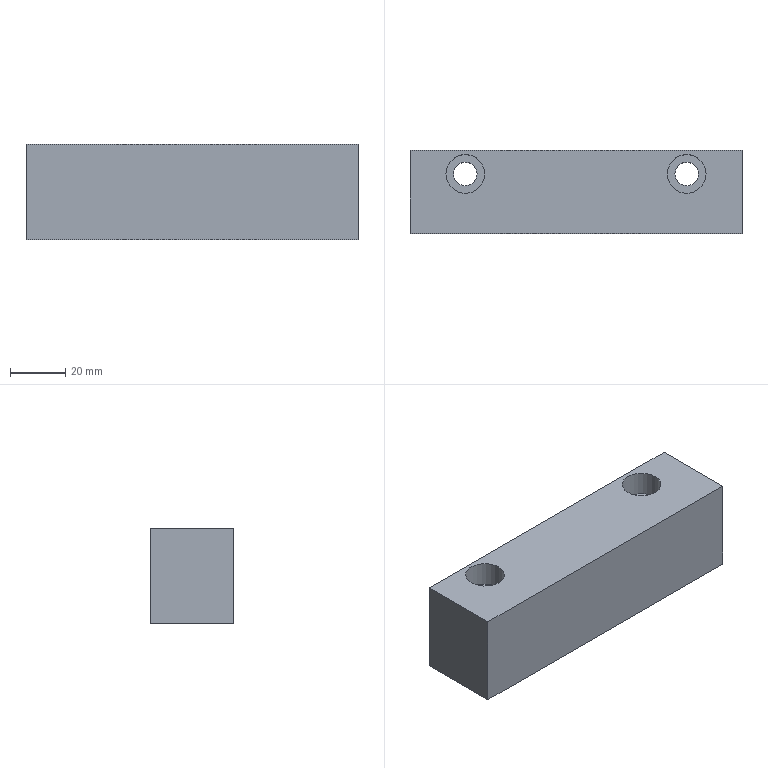Part | NX | features solid 2 | 1 solid | 12 faces | box 120 x 30 x 34.5 mm | volume 118535 mm3 | plane 8 | cylinder 4 | commonest cylinder face diameters 8.5 x2 14 x2
STEP:
#1=CARTESIAN_POINT('',(-55.,85.,-35.));
#2=VERTEX_POINT('',#1);
#3=CARTESIAN_POINT('',(-55.,115.,-35.));
#4=VERTEX_POINT('',#3);
#5=CARTESIAN_POINT('',(-55.,92.5,-35.));
#6=DIRECTION('',(0.,1.,0.));
#7=VECTOR('',#6,1000.);
#8=LINE('',#5,#7);
#9=EDGE_CURVE('',#2,#4,#8,.T.);
#10=ORIENTED_EDGE('',*,*,#9,.F.);
#11=CARTESIAN_POINT('',(-175.,85.,-35.));
#12=VERTEX_POINT('',#11);
#13=CARTESIAN_POINT('',(-90.,85.,-35.));
#14=DIRECTION('',(1.,0.,0.));
#15=VECTOR('',#14,1000.);
#16=LINE('',#13,#15);
#17=EDGE_CURVE('',#12,#2,#16,.T.);
#18=ORIENTED_EDGE('',*,*,#17,.F.);
#19=CARTESIAN_POINT('',(-175.,115.,-35.));
#20=VERTEX_POINT('',#19);
#21=CARTESIAN_POINT('',(-175.,0.,-35.));
#22=DIRECTION('',(0.,-1.,0.));
#23=VECTOR('',#22,1000.);
#24=LINE('',#21,#23);
#25=EDGE_CURVE('',#20,#12,#24,.T.);
#26=ORIENTED_EDGE('',*,*,#25,.F.);
#27=CARTESIAN_POINT('',(-90.,115.,-35.));
#28=DIRECTION('',(-1.,0.,0.));
#29=VECTOR('',#28,1000.);
#30=LINE('',#27,#29);
#31=EDGE_CURVE('',#4,#20,#30,.T.);
#32=ORIENTED_EDGE('',*,*,#31,.F.);
#33=EDGE_LOOP('',(#10,#18,#26,#32));
#34=FACE_BOUND('',#33,.T.);
#35=CARTESIAN_POINT('',(-150.75,106.5,-35.));
#36=VERTEX_POINT('',#35);
#37=CARTESIAN_POINT('',(-155.,106.5,-35.));
#38=DIRECTION('',(0.,0.,1.));
#39=DIRECTION('',(1.,0.,0.));
#40=AXIS2_PLACEMENT_3D('',#37,#38,#39);
#41=CIRCLE('',#40,4.25);
#42=EDGE_CURVE('',#36,#36,#41,.T.);
#43=ORIENTED_EDGE('',*,*,#42,.T.);
#44=EDGE_LOOP('',(#43));
#45=FACE_BOUND('',#44,.T.);
#46=CARTESIAN_POINT('',(-70.75,106.5,-35.));
#47=VERTEX_POINT('',#46);
#48=CARTESIAN_POINT('',(-75.,106.5,-35.));
#49=DIRECTION('',(0.,0.,1.));
#50=DIRECTION('',(1.,0.,0.));
#51=AXIS2_PLACEMENT_3D('',#48,#49,#50);
#52=CIRCLE('',#51,4.25);
#53=EDGE_CURVE('',#47,#47,#52,.T.);
#54=ORIENTED_EDGE('',*,*,#53,.T.);
#55=EDGE_LOOP('',(#54));
#56=FACE_BOUND('',#55,.T.);
#57=CARTESIAN_POINT('',(-90.,92.5,-35.));
#58=DIRECTION('',(0.,0.,-1.));
#59=DIRECTION('',(-1.,0.,0.));
#60=AXIS2_PLACEMENT_3D('',#57,#58,#59);
#61=PLANE('',#60);
#62=ADVANCED_FACE('',(#34,#45,#56),#61,.T.);
#63=CARTESIAN_POINT('',(-55.,85.,-0.5));
#64=VERTEX_POINT('',#63);
#65=CARTESIAN_POINT('',(-55.,85.,-40.));
#66=DIRECTION('',(0.,0.,1.));
#67=VECTOR('',#66,1000.);
#68=LINE('',#65,#67);
#69=EDGE_CURVE('',#2,#64,#68,.T.);
#70=ORIENTED_EDGE('',*,*,#69,.F.);
#71=ORIENTED_EDGE('',*,*,#9,.T.);
#72=CARTESIAN_POINT('',(-55.,115.,-0.5));
#73=VERTEX_POINT('',#72);
#74=CARTESIAN_POINT('',(-55.,115.,-40.));
#75=DIRECTION('',(0.,0.,1.));
#76=VECTOR('',#75,1000.);
#77=LINE('',#74,#76);
#78=EDGE_CURVE('',#4,#73,#77,.T.);
#79=ORIENTED_EDGE('',*,*,#78,.T.);
#80=CARTESIAN_POINT('',(-55.,92.5,-0.5));
#81=DIRECTION('',(0.,-1.,0.));
#82=VECTOR('',#81,1000.);
#83=LINE('',#80,#82);
#84=EDGE_CURVE('',#73,#64,#83,.T.);
#85=ORIENTED_EDGE('',*,*,#84,.T.);
#86=EDGE_LOOP('',(#70,#71,#79,#85));
#87=FACE_BOUND('',#86,.T.);
#88=CARTESIAN_POINT('',(-55.,92.5,-40.));
#89=DIRECTION('',(1.,0.,0.));
#90=DIRECTION('',(0.,0.,-1.));
#91=AXIS2_PLACEMENT_3D('',#88,#89,#90);
#92=PLANE('',#91);
#93=ADVANCED_FACE('',(#87),#92,.T.);
#94=CARTESIAN_POINT('',(-68.,106.5,-0.5));
#95=VERTEX_POINT('',#94);
#96=CARTESIAN_POINT('',(-75.,106.5,-0.5));
#97=DIRECTION('',(0.,0.,-1.));
#98=DIRECTION('',(1.,0.,0.));
#99=AXIS2_PLACEMENT_3D('',#96,#97,#98);
#100=CIRCLE('',#99,7.);
#101=EDGE_CURVE('',#95,#95,#100,.T.);
#102=ORIENTED_EDGE('',*,*,#101,.T.);
#103=EDGE_LOOP('',(#102));
#104=FACE_BOUND('',#103,.T.);
#105=ORIENTED_EDGE('',*,*,#84,.F.);
#106=CARTESIAN_POINT('',(-175.,115.,-0.5));
#107=VERTEX_POINT('',#106);
#108=CARTESIAN_POINT('',(-90.,115.,-0.5));
#109=DIRECTION('',(1.,0.,0.));
#110=VECTOR('',#109,1000.);
#111=LINE('',#108,#110);
#112=EDGE_CURVE('',#107,#73,#111,.T.);
#113=ORIENTED_EDGE('',*,*,#112,.F.);
#114=CARTESIAN_POINT('',(-175.,85.,-0.5));
#115=VERTEX_POINT('',#114);
#116=CARTESIAN_POINT('',(-175.,0.,-0.5));
#117=DIRECTION('',(0.,1.,0.));
#118=VECTOR('',#117,1000.);
#119=LINE('',#116,#118);
#120=EDGE_CURVE('',#115,#107,#119,.T.);
#121=ORIENTED_EDGE('',*,*,#120,.F.);
#122=CARTESIAN_POINT('',(-90.,85.,-0.5));
#123=DIRECTION('',(-1.,0.,0.));
#124=VECTOR('',#123,1000.);
#125=LINE('',#122,#124);
#126=EDGE_CURVE('',#64,#115,#125,.T.);
#127=ORIENTED_EDGE('',*,*,#126,.F.);
#128=EDGE_LOOP('',(#105,#113,#121,#127));
#129=FACE_BOUND('',#128,.T.);
#130=CARTESIAN_POINT('',(-148.,106.5,-0.5));
#131=VERTEX_POINT('',#130);
#132=CARTESIAN_POINT('',(-155.,106.5,-0.5));
#133=DIRECTION('',(0.,0.,-1.));
#134=DIRECTION('',(1.,0.,0.));
#135=AXIS2_PLACEMENT_3D('',#132,#133,#134);
#136=CIRCLE('',#135,7.);
#137=EDGE_CURVE('',#131,#131,#136,.T.);
#138=ORIENTED_EDGE('',*,*,#137,.T.);
#139=EDGE_LOOP('',(#138));
#140=FACE_BOUND('',#139,.T.);
#141=CARTESIAN_POINT('',(0.,0.,-0.5));
#142=DIRECTION('',(0.,0.,1.));
#143=DIRECTION('',(1.,0.,0.));
#144=AXIS2_PLACEMENT_3D('',#141,#142,#143);
#145=PLANE('',#144);
#146=ADVANCED_FACE('',(#104,#129,#140),#145,.T.);
#147=ORIENTED_EDGE('',*,*,#17,.T.);
#148=ORIENTED_EDGE('',*,*,#69,.T.);
#149=ORIENTED_EDGE('',*,*,#126,.T.);
#150=CARTESIAN_POINT('',(-175.,85.,-110.5));
#151=DIRECTION('',(0.,0.,1.));
#152=VECTOR('',#151,1000.);
#153=LINE('',#150,#152);
#154=EDGE_CURVE('',#12,#115,#153,.T.);
#155=ORIENTED_EDGE('',*,*,#154,.F.);
#156=EDGE_LOOP('',(#147,#148,#149,#155));
#157=FACE_BOUND('',#156,.T.);
#158=CARTESIAN_POINT('',(-90.,85.,-40.));
#159=DIRECTION('',(0.,-1.,0.));
#160=DIRECTION('',(0.,0.,-1.));
#161=AXIS2_PLACEMENT_3D('',#158,#159,#160);
#162=PLANE('',#161);
#163=ADVANCED_FACE('',(#157),#162,.T.);
#164=ORIENTED_EDGE('',*,*,#154,.T.);
#165=ORIENTED_EDGE('',*,*,#120,.T.);
#166=CARTESIAN_POINT('',(-175.,115.,-40.));
#167=DIRECTION('',(0.,0.,1.));
#168=VECTOR('',#167,1000.);
#169=LINE('',#166,#168);
#170=EDGE_CURVE('',#20,#107,#169,.T.);
#171=ORIENTED_EDGE('',*,*,#170,.F.);
#172=ORIENTED_EDGE('',*,*,#25,.T.);
#173=EDGE_LOOP('',(#164,#165,#171,#172));
#174=FACE_BOUND('',#173,.T.);
#175=CARTESIAN_POINT('',(-175.,0.,-110.5));
#176=DIRECTION('',(-1.,0.,0.));
#177=DIRECTION('',(0.,0.,1.));
#178=AXIS2_PLACEMENT_3D('',#175,#176,#177);
#179=PLANE('',#178);
#180=ADVANCED_FACE('',(#174),#179,.T.);
#181=ORIENTED_EDGE('',*,*,#112,.T.);
#182=ORIENTED_EDGE('',*,*,#78,.F.);
#183=ORIENTED_EDGE('',*,*,#31,.T.);
#184=ORIENTED_EDGE('',*,*,#170,.T.);
#185=EDGE_LOOP('',(#181,#182,#183,#184));
#186=FACE_BOUND('',#185,.T.);
#187=CARTESIAN_POINT('',(-90.,115.,-40.));
#188=DIRECTION('',(0.,1.,0.));
#189=DIRECTION('',(0.,0.,1.));
#190=AXIS2_PLACEMENT_3D('',#187,#188,#189);
#191=PLANE('',#190);
#192=ADVANCED_FACE('',(#186),#191,.T.);
#193=CARTESIAN_POINT('',(-79.25,106.5,-9.5));
#194=VERTEX_POINT('',#193);
#195=CARTESIAN_POINT('',(-75.,106.5,-9.5));
#196=DIRECTION('',(0.,0.,-1.));
#197=DIRECTION('',(-1.,0.,0.));
#198=AXIS2_PLACEMENT_3D('',#195,#196,#197);
#199=CIRCLE('',#198,4.25);
#200=EDGE_CURVE('',#194,#194,#199,.F.);
#201=ORIENTED_EDGE('',*,*,#200,.F.);
#202=EDGE_LOOP('',(#201));
#203=FACE_BOUND('',#202,.T.);
#204=CARTESIAN_POINT('',(-68.,106.5,-9.5));
#205=VERTEX_POINT('',#204);
#206=CARTESIAN_POINT('',(-75.,106.5,-9.5));
#207=DIRECTION('',(0.,0.,1.));
#208=DIRECTION('',(1.,0.,0.));
#209=AXIS2_PLACEMENT_3D('',#206,#207,#208);
#210=CIRCLE('',#209,7.);
#211=EDGE_CURVE('',#205,#205,#210,.F.);
#212=ORIENTED_EDGE('',*,*,#211,.F.);
#213=EDGE_LOOP('',(#212));
#214=FACE_BOUND('',#213,.T.);
#215=CARTESIAN_POINT('',(-75.,106.5,-9.5));
#216=DIRECTION('',(0.,0.,-1.));
#217=DIRECTION('',(-1.,0.,0.));
#218=AXIS2_PLACEMENT_3D('',#215,#216,#217);
#219=PLANE('',#218);
#220=ADVANCED_FACE('',(#203,#214),#219,.F.);
#221=ORIENTED_EDGE('',*,*,#211,.T.);
#222=EDGE_LOOP('',(#221));
#223=FACE_BOUND('',#222,.T.);
#224=ORIENTED_EDGE('',*,*,#101,.F.);
#225=EDGE_LOOP('',(#224));
#226=FACE_BOUND('',#225,.T.);
#227=CARTESIAN_POINT('',(-75.,106.5,-0.5));
#228=DIRECTION('',(0.,0.,-1.));
#229=DIRECTION('',(1.,0.,0.));
#230=AXIS2_PLACEMENT_3D('',#227,#228,#229);
#231=CYLINDRICAL_SURFACE('',#230,7.);
#232=ADVANCED_FACE('',(#223,#226),#231,.F.);
#233=ORIENTED_EDGE('',*,*,#200,.T.);
#234=EDGE_LOOP('',(#233));
#235=FACE_BOUND('',#234,.T.);
#236=ORIENTED_EDGE('',*,*,#53,.F.);
#237=EDGE_LOOP('',(#236));
#238=FACE_BOUND('',#237,.T.);
#239=CARTESIAN_POINT('',(-75.,106.5,-0.5));
#240=DIRECTION('',(0.,0.,-1.));
#241=DIRECTION('',(1.,0.,0.));
#242=AXIS2_PLACEMENT_3D('',#239,#240,#241);
#243=CYLINDRICAL_SURFACE('',#242,4.25);
#244=ADVANCED_FACE('',(#235,#238),#243,.F.);
#245=CARTESIAN_POINT('',(-159.25,106.5,-9.5));
#246=VERTEX_POINT('',#245);
#247=CARTESIAN_POINT('',(-155.,106.5,-9.5));
#248=DIRECTION('',(0.,0.,-1.));
#249=DIRECTION('',(-1.,0.,0.));
#250=AXIS2_PLACEMENT_3D('',#247,#248,#249);
#251=CIRCLE('',#250,4.25);
#252=EDGE_CURVE('',#246,#246,#251,.F.);
#253=ORIENTED_EDGE('',*,*,#252,.F.);
#254=EDGE_LOOP('',(#253));
#255=FACE_BOUND('',#254,.T.);
#256=CARTESIAN_POINT('',(-148.,106.5,-9.5));
#257=VERTEX_POINT('',#256);
#258=CARTESIAN_POINT('',(-155.,106.5,-9.5));
#259=DIRECTION('',(0.,0.,1.));
#260=DIRECTION('',(1.,0.,0.));
#261=AXIS2_PLACEMENT_3D('',#258,#259,#260);
#262=CIRCLE('',#261,7.);
#263=EDGE_CURVE('',#257,#257,#262,.F.);
#264=ORIENTED_EDGE('',*,*,#263,.F.);
#265=EDGE_LOOP('',(#264));
#266=FACE_BOUND('',#265,.T.);
#267=CARTESIAN_POINT('',(-155.,106.5,-9.5));
#268=DIRECTION('',(0.,0.,-1.));
#269=DIRECTION('',(-1.,0.,0.));
#270=AXIS2_PLACEMENT_3D('',#267,#268,#269);
#271=PLANE('',#270);
#272=ADVANCED_FACE('',(#255,#266),#271,.F.);
#273=ORIENTED_EDGE('',*,*,#263,.T.);
#274=EDGE_LOOP('',(#273));
#275=FACE_BOUND('',#274,.T.);
#276=ORIENTED_EDGE('',*,*,#137,.F.);
#277=EDGE_LOOP('',(#276));
#278=FACE_BOUND('',#277,.T.);
#279=CARTESIAN_POINT('',(-155.,106.5,-0.5));
#280=DIRECTION('',(0.,0.,-1.));
#281=DIRECTION('',(1.,0.,0.));
#282=AXIS2_PLACEMENT_3D('',#279,#280,#281);
#283=CYLINDRICAL_SURFACE('',#282,7.);
#284=ADVANCED_FACE('',(#275,#278),#283,.F.);
#285=ORIENTED_EDGE('',*,*,#252,.T.);
#286=EDGE_LOOP('',(#285));
#287=FACE_BOUND('',#286,.T.);
#288=ORIENTED_EDGE('',*,*,#42,.F.);
#289=EDGE_LOOP('',(#288));
#290=FACE_BOUND('',#289,.T.);
#291=CARTESIAN_POINT('',(-155.,106.5,-0.5));
#292=DIRECTION('',(0.,0.,-1.));
#293=DIRECTION('',(1.,0.,0.));
#294=AXIS2_PLACEMENT_3D('',#291,#292,#293);
#295=CYLINDRICAL_SURFACE('',#294,4.25);
#296=ADVANCED_FACE('',(#287,#290),#295,.F.);
#297=CLOSED_SHELL('',(#62,#93,#146,#163,#180,#192,#220,#232,#244,#272,#284,#296));
#298=MANIFOLD_SOLID_BREP('',#297);
#299=(LENGTH_UNIT()NAMED_UNIT(*)SI_UNIT(.MILLI.,.METRE.));
#300=UNCERTAINTY_MEASURE_WITH_UNIT(LENGTH_MEASURE(0.00001),#299,'','');
#301=(NAMED_UNIT(*)PLANE_ANGLE_UNIT()SI_UNIT($,.RADIAN.));
#302=(NAMED_UNIT(*)SI_UNIT($,.STERADIAN.)SOLID_ANGLE_UNIT());
#303=(GEOMETRIC_REPRESENTATION_CONTEXT(3)GLOBAL_UNCERTAINTY_ASSIGNED_CONTEXT((#300))GLOBAL_UNIT_ASSIGNED_CONTEXT((#299,#301,#302))REPRESENTATION_CONTEXT('',''));
#304=ADVANCED_BREP_SHAPE_REPRESENTATION('',(#298),#303);